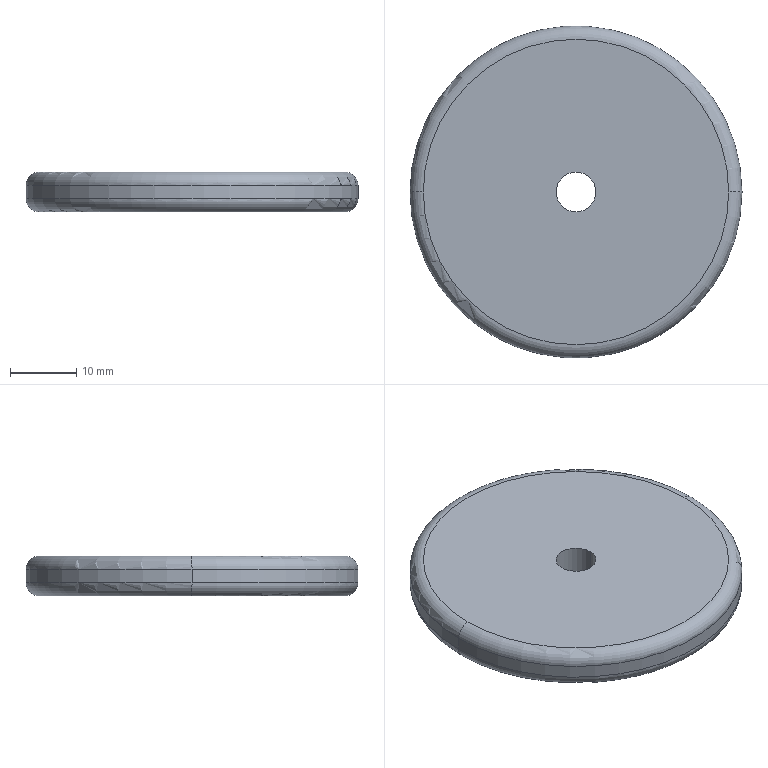Part | SolidWorks | features Extrusion 1, Fillet 1 | 1 solid | 10 faces | box 50 x 50 x 6 mm | volume 11346 mm3 | torus 4 | cylinder 4 | plane 2 | commonest cylinder face diameters 6 x2 50 x2
STEP:
#1=CARTESIAN_POINT('',(-49.873,-17.895,0.));
#2=VERTEX_POINT('',#1);
#3=CARTESIAN_POINT('',(-3.873,-17.895,0.));
#4=VERTEX_POINT('',#3);
#5=CARTESIAN_POINT('',(-26.873,-17.895,0.));
#6=DIRECTION('',(0.,0.,-1.));
#7=DIRECTION('',(1.,0.,0.));
#8=AXIS2_PLACEMENT_3D('',#5,#6,#7);
#9=CIRCLE('',#8,23.);
#10=EDGE_CURVE('',#2,#4,#9,.T.);
#11=ORIENTED_EDGE('',*,*,#10,.F.);
#12=CARTESIAN_POINT('',(-51.873,-17.895,2.));
#13=VERTEX_POINT('',#12);
#14=CARTESIAN_POINT('',(-49.873,-17.895,2.));
#15=DIRECTION('',(0.,1.,0.));
#16=DIRECTION('',(-1.,0.,0.));
#17=AXIS2_PLACEMENT_3D('',#14,#15,#16);
#18=CIRCLE('',#17,2.);
#19=EDGE_CURVE('',#2,#13,#18,.T.);
#20=ORIENTED_EDGE('',*,*,#19,.T.);
#21=CARTESIAN_POINT('',(-1.873,-17.895,2.));
#22=VERTEX_POINT('',#21);
#23=CARTESIAN_POINT('',(-26.873,-17.895,2.));
#24=DIRECTION('',(0.,0.,1.));
#25=DIRECTION('',(1.,0.,0.));
#26=AXIS2_PLACEMENT_3D('',#23,#24,#25);
#27=CIRCLE('',#26,25.);
#28=EDGE_CURVE('',#22,#13,#27,.T.);
#29=ORIENTED_EDGE('',*,*,#28,.F.);
#30=CARTESIAN_POINT('',(-3.873,-17.895,2.));
#31=DIRECTION('',(0.,-1.,0.));
#32=DIRECTION('',(0.,0.,-1.));
#33=AXIS2_PLACEMENT_3D('',#30,#31,#32);
#34=CIRCLE('',#33,2.);
#35=EDGE_CURVE('',#4,#22,#34,.T.);
#36=ORIENTED_EDGE('',*,*,#35,.F.);
#37=EDGE_LOOP('',(#11,#20,#29,#36));
#38=FACE_OUTER_BOUND('',#37,.T.);
#39=CARTESIAN_POINT('',(-26.873,-17.895,2.));
#40=DIRECTION('',(0.,0.,1.));
#41=DIRECTION('',(1.,0.,0.));
#42=AXIS2_PLACEMENT_3D('',#39,#40,#41);
#43=TOROIDAL_SURFACE('',#42,23.,2.);
#44=ADVANCED_FACE('',(#38),#43,.T.);
#45=CARTESIAN_POINT('',(-51.873,-17.895,4.));
#46=VERTEX_POINT('',#45);
#47=CARTESIAN_POINT('',(-1.873,-17.895,4.));
#48=VERTEX_POINT('',#47);
#49=CARTESIAN_POINT('',(-26.873,-17.895,4.));
#50=DIRECTION('',(0.,0.,-1.));
#51=DIRECTION('',(1.,0.,0.));
#52=AXIS2_PLACEMENT_3D('',#49,#50,#51);
#53=CIRCLE('',#52,25.);
#54=EDGE_CURVE('',#46,#48,#53,.T.);
#55=ORIENTED_EDGE('',*,*,#54,.F.);
#56=CARTESIAN_POINT('',(-49.873,-17.895,6.));
#57=VERTEX_POINT('',#56);
#58=CARTESIAN_POINT('',(-49.873,-17.895,4.));
#59=DIRECTION('',(0.,1.,0.));
#60=DIRECTION('',(-1.,0.,0.));
#61=AXIS2_PLACEMENT_3D('',#58,#59,#60);
#62=CIRCLE('',#61,2.);
#63=EDGE_CURVE('',#46,#57,#62,.T.);
#64=ORIENTED_EDGE('',*,*,#63,.T.);
#65=CARTESIAN_POINT('',(-3.873,-17.895,6.));
#66=VERTEX_POINT('',#65);
#67=CARTESIAN_POINT('',(-26.873,-17.895,6.));
#68=DIRECTION('',(0.,0.,1.));
#69=DIRECTION('',(1.,0.,0.));
#70=AXIS2_PLACEMENT_3D('',#67,#68,#69);
#71=CIRCLE('',#70,23.);
#72=EDGE_CURVE('',#66,#57,#71,.T.);
#73=ORIENTED_EDGE('',*,*,#72,.F.);
#74=CARTESIAN_POINT('',(-3.873,-17.895,4.));
#75=DIRECTION('',(0.,-1.,0.));
#76=DIRECTION('',(0.,0.,-1.));
#77=AXIS2_PLACEMENT_3D('',#74,#75,#76);
#78=CIRCLE('',#77,2.);
#79=EDGE_CURVE('',#48,#66,#78,.T.);
#80=ORIENTED_EDGE('',*,*,#79,.F.);
#81=EDGE_LOOP('',(#55,#64,#73,#80));
#82=FACE_OUTER_BOUND('',#81,.T.);
#83=CARTESIAN_POINT('',(-26.873,-17.895,4.));
#84=DIRECTION('',(0.,0.,1.));
#85=DIRECTION('',(1.,0.,0.));
#86=AXIS2_PLACEMENT_3D('',#83,#84,#85);
#87=TOROIDAL_SURFACE('',#86,23.,2.);
#88=ADVANCED_FACE('',(#82),#87,.T.);
#89=CARTESIAN_POINT('',(-29.873,-17.895,6.));
#90=VERTEX_POINT('',#89);
#91=CARTESIAN_POINT('',(-23.873,-17.895,6.));
#92=VERTEX_POINT('',#91);
#93=CARTESIAN_POINT('',(-26.873,-17.895,6.));
#94=DIRECTION('',(0.,0.,1.));
#95=DIRECTION('',(1.,0.,0.));
#96=AXIS2_PLACEMENT_3D('',#93,#94,#95);
#97=CIRCLE('',#96,3.);
#98=EDGE_CURVE('',#90,#92,#97,.T.);
#99=ORIENTED_EDGE('',*,*,#98,.T.);
#100=CARTESIAN_POINT('',(-23.873,-17.895,0.));
#101=VERTEX_POINT('',#100);
#102=CARTESIAN_POINT('',(-23.873,-17.895,6.));
#103=DIRECTION('',(0.,0.,-1.));
#104=VECTOR('',#103,1000.);
#105=LINE('',#102,#104);
#106=EDGE_CURVE('',#92,#101,#105,.T.);
#107=ORIENTED_EDGE('',*,*,#106,.T.);
#108=CARTESIAN_POINT('',(-29.873,-17.895,0.));
#109=VERTEX_POINT('',#108);
#110=CARTESIAN_POINT('',(-26.873,-17.895,0.));
#111=DIRECTION('',(0.,0.,1.));
#112=DIRECTION('',(1.,0.,0.));
#113=AXIS2_PLACEMENT_3D('',#110,#111,#112);
#114=CIRCLE('',#113,3.);
#115=EDGE_CURVE('',#109,#101,#114,.T.);
#116=ORIENTED_EDGE('',*,*,#115,.F.);
#117=CARTESIAN_POINT('',(-29.873,-17.895,6.));
#118=DIRECTION('',(0.,0.,-1.));
#119=VECTOR('',#118,1000.);
#120=LINE('',#117,#119);
#121=EDGE_CURVE('',#90,#109,#120,.T.);
#122=ORIENTED_EDGE('',*,*,#121,.F.);
#123=EDGE_LOOP('',(#99,#107,#116,#122));
#124=FACE_OUTER_BOUND('',#123,.T.);
#125=CARTESIAN_POINT('',(-26.873,-17.895,6.));
#126=DIRECTION('',(0.,0.,-1.));
#127=DIRECTION('',(-1.,0.,0.));
#128=AXIS2_PLACEMENT_3D('',#125,#126,#127);
#129=CYLINDRICAL_SURFACE('',#128,3.);
#130=ADVANCED_FACE('',(#124),#129,.F.);
#131=ORIENTED_EDGE('',*,*,#54,.T.);
#132=CARTESIAN_POINT('',(-1.873,-17.895,6.));
#133=DIRECTION('',(0.,0.,-1.));
#134=VECTOR('',#133,1000.);
#135=LINE('',#132,#134);
#136=EDGE_CURVE('',#48,#22,#135,.T.);
#137=ORIENTED_EDGE('',*,*,#136,.T.);
#138=ORIENTED_EDGE('',*,*,#28,.T.);
#139=CARTESIAN_POINT('',(-51.873,-17.895,6.));
#140=DIRECTION('',(0.,0.,-1.));
#141=VECTOR('',#140,1000.);
#142=LINE('',#139,#141);
#143=EDGE_CURVE('',#46,#13,#142,.T.);
#144=ORIENTED_EDGE('',*,*,#143,.F.);
#145=EDGE_LOOP('',(#131,#137,#138,#144));
#146=FACE_OUTER_BOUND('',#145,.T.);
#147=CARTESIAN_POINT('',(-26.873,-17.895,6.));
#148=DIRECTION('',(0.,0.,-1.));
#149=DIRECTION('',(-1.,0.,0.));
#150=AXIS2_PLACEMENT_3D('',#147,#148,#149);
#151=CYLINDRICAL_SURFACE('',#150,25.);
#152=ADVANCED_FACE('',(#146),#151,.T.);
#153=ORIENTED_EDGE('',*,*,#72,.T.);
#154=CARTESIAN_POINT('',(-26.873,-17.895,6.));
#155=DIRECTION('',(0.,0.,1.));
#156=DIRECTION('',(1.,0.,0.));
#157=AXIS2_PLACEMENT_3D('',#154,#155,#156);
#158=CIRCLE('',#157,23.);
#159=EDGE_CURVE('',#57,#66,#158,.T.);
#160=ORIENTED_EDGE('',*,*,#159,.T.);
#161=EDGE_LOOP('',(#153,#160));
#162=FACE_OUTER_BOUND('',#161,.T.);
#163=ORIENTED_EDGE('',*,*,#98,.F.);
#164=CARTESIAN_POINT('',(-26.873,-17.895,6.));
#165=DIRECTION('',(0.,0.,1.));
#166=DIRECTION('',(1.,0.,0.));
#167=AXIS2_PLACEMENT_3D('',#164,#165,#166);
#168=CIRCLE('',#167,3.);
#169=EDGE_CURVE('',#92,#90,#168,.T.);
#170=ORIENTED_EDGE('',*,*,#169,.F.);
#171=EDGE_LOOP('',(#163,#170));
#172=FACE_BOUND('',#171,.T.);
#173=CARTESIAN_POINT('',(-26.873,-17.895,6.));
#174=DIRECTION('',(0.,0.,1.));
#175=DIRECTION('',(1.,0.,0.));
#176=AXIS2_PLACEMENT_3D('',#173,#174,#175);
#177=PLANE('',#176);
#178=ADVANCED_FACE('',(#162,#172),#177,.T.);
#179=CARTESIAN_POINT('',(-26.873,-17.895,0.));
#180=DIRECTION('',(0.,0.,-1.));
#181=DIRECTION('',(1.,0.,0.));
#182=AXIS2_PLACEMENT_3D('',#179,#180,#181);
#183=CIRCLE('',#182,23.);
#184=EDGE_CURVE('',#4,#2,#183,.T.);
#185=ORIENTED_EDGE('',*,*,#184,.T.);
#186=ORIENTED_EDGE('',*,*,#10,.T.);
#187=EDGE_LOOP('',(#185,#186));
#188=FACE_OUTER_BOUND('',#187,.T.);
#189=ORIENTED_EDGE('',*,*,#115,.T.);
#190=CARTESIAN_POINT('',(-26.873,-17.895,0.));
#191=DIRECTION('',(0.,0.,1.));
#192=DIRECTION('',(1.,0.,0.));
#193=AXIS2_PLACEMENT_3D('',#190,#191,#192);
#194=CIRCLE('',#193,3.);
#195=EDGE_CURVE('',#101,#109,#194,.T.);
#196=ORIENTED_EDGE('',*,*,#195,.T.);
#197=EDGE_LOOP('',(#189,#196));
#198=FACE_BOUND('',#197,.T.);
#199=CARTESIAN_POINT('',(-26.873,-17.895,0.));
#200=DIRECTION('',(0.,0.,1.));
#201=DIRECTION('',(1.,0.,0.));
#202=AXIS2_PLACEMENT_3D('',#199,#200,#201);
#203=PLANE('',#202);
#204=ADVANCED_FACE('',(#188,#198),#203,.F.);
#205=ORIENTED_EDGE('',*,*,#136,.F.);
#206=CARTESIAN_POINT('',(-26.873,-17.895,4.));
#207=DIRECTION('',(0.,0.,-1.));
#208=DIRECTION('',(1.,0.,0.));
#209=AXIS2_PLACEMENT_3D('',#206,#207,#208);
#210=CIRCLE('',#209,25.);
#211=EDGE_CURVE('',#48,#46,#210,.T.);
#212=ORIENTED_EDGE('',*,*,#211,.T.);
#213=ORIENTED_EDGE('',*,*,#143,.T.);
#214=CARTESIAN_POINT('',(-26.873,-17.895,2.));
#215=DIRECTION('',(0.,0.,1.));
#216=DIRECTION('',(1.,0.,0.));
#217=AXIS2_PLACEMENT_3D('',#214,#215,#216);
#218=CIRCLE('',#217,25.);
#219=EDGE_CURVE('',#13,#22,#218,.T.);
#220=ORIENTED_EDGE('',*,*,#219,.T.);
#221=EDGE_LOOP('',(#205,#212,#213,#220));
#222=FACE_OUTER_BOUND('',#221,.T.);
#223=CARTESIAN_POINT('',(-26.873,-17.895,6.));
#224=DIRECTION('',(0.,0.,-1.));
#225=DIRECTION('',(-1.,0.,0.));
#226=AXIS2_PLACEMENT_3D('',#223,#224,#225);
#227=CYLINDRICAL_SURFACE('',#226,25.);
#228=ADVANCED_FACE('',(#222),#227,.T.);
#229=ORIENTED_EDGE('',*,*,#106,.F.);
#230=ORIENTED_EDGE('',*,*,#169,.T.);
#231=ORIENTED_EDGE('',*,*,#121,.T.);
#232=ORIENTED_EDGE('',*,*,#195,.F.);
#233=EDGE_LOOP('',(#229,#230,#231,#232));
#234=FACE_OUTER_BOUND('',#233,.T.);
#235=CARTESIAN_POINT('',(-26.873,-17.895,6.));
#236=DIRECTION('',(0.,0.,-1.));
#237=DIRECTION('',(-1.,0.,0.));
#238=AXIS2_PLACEMENT_3D('',#235,#236,#237);
#239=CYLINDRICAL_SURFACE('',#238,3.);
#240=ADVANCED_FACE('',(#234),#239,.F.);
#241=ORIENTED_EDGE('',*,*,#63,.F.);
#242=ORIENTED_EDGE('',*,*,#211,.F.);
#243=ORIENTED_EDGE('',*,*,#79,.T.);
#244=ORIENTED_EDGE('',*,*,#159,.F.);
#245=EDGE_LOOP('',(#241,#242,#243,#244));
#246=FACE_OUTER_BOUND('',#245,.T.);
#247=CARTESIAN_POINT('',(-26.873,-17.895,4.));
#248=DIRECTION('',(0.,0.,1.));
#249=DIRECTION('',(1.,0.,0.));
#250=AXIS2_PLACEMENT_3D('',#247,#248,#249);
#251=TOROIDAL_SURFACE('',#250,23.,2.);
#252=ADVANCED_FACE('',(#246),#251,.T.);
#253=ORIENTED_EDGE('',*,*,#19,.F.);
#254=ORIENTED_EDGE('',*,*,#184,.F.);
#255=ORIENTED_EDGE('',*,*,#35,.T.);
#256=ORIENTED_EDGE('',*,*,#219,.F.);
#257=EDGE_LOOP('',(#253,#254,#255,#256));
#258=FACE_OUTER_BOUND('',#257,.T.);
#259=CARTESIAN_POINT('',(-26.873,-17.895,2.));
#260=DIRECTION('',(0.,0.,1.));
#261=DIRECTION('',(1.,0.,0.));
#262=AXIS2_PLACEMENT_3D('',#259,#260,#261);
#263=TOROIDAL_SURFACE('',#262,23.,2.);
#264=ADVANCED_FACE('',(#258),#263,.T.);
#265=CLOSED_SHELL('',(#44,#88,#130,#152,#178,#204,#228,#240,#252,#264));
#266=MANIFOLD_SOLID_BREP('',#265);
#267=CARTESIAN_POINT('',(0.,0.,0.));
#268=DIRECTION('',(0.,0.,1.));
#269=DIRECTION('',(1.,0.,0.));
#270=AXIS2_PLACEMENT_3D('',#267,#268,#269);
#271=(LENGTH_UNIT()NAMED_UNIT(*)SI_UNIT(.MILLI.,.METRE.));
#272=UNCERTAINTY_MEASURE_WITH_UNIT(LENGTH_MEASURE(0.00001),#271,'','');
#273=(NAMED_UNIT(*)PLANE_ANGLE_UNIT()SI_UNIT($,.RADIAN.));
#274=(NAMED_UNIT(*)SI_UNIT($,.STERADIAN.)SOLID_ANGLE_UNIT());
#275=(GEOMETRIC_REPRESENTATION_CONTEXT(3)GLOBAL_UNCERTAINTY_ASSIGNED_CONTEXT((#272))GLOBAL_UNIT_ASSIGNED_CONTEXT((#271,#273,#274))REPRESENTATION_CONTEXT('',''));
#276=ADVANCED_BREP_SHAPE_REPRESENTATION('',(#266,#270),#275);